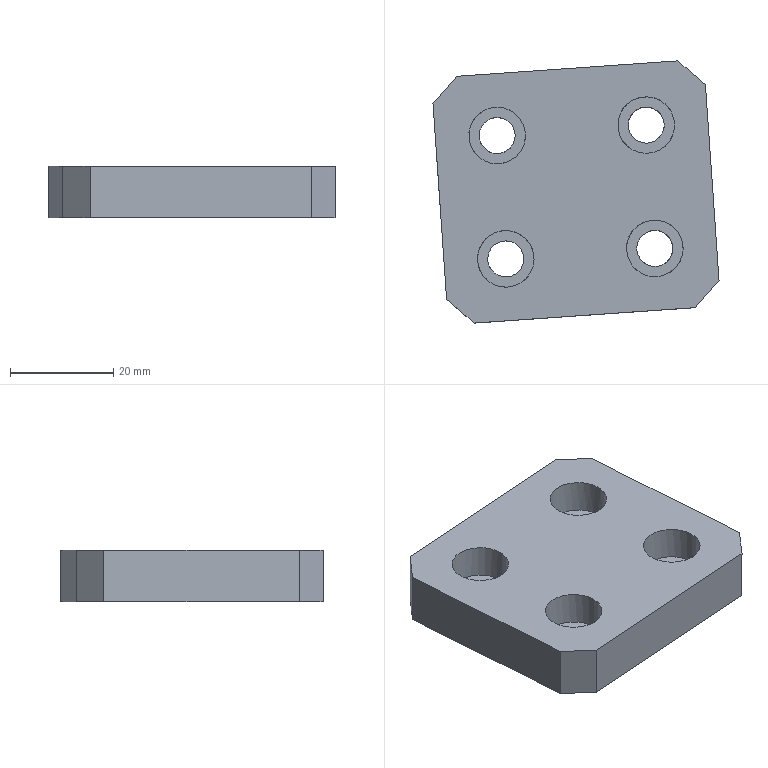Part | STEP file | 车灯-后视镜_id658_x_t | 1 solid | 22 faces | box 55.522 x 50.883 x 10 mm | volume 21930 mm3 | plane 14 | cylinder 8 | commonest cylinder face diameters 7 x4 11 x4
STEP:
#1=CARTESIAN_POINT('',(-17.129,7.094,-255.5));
#2=VERTEX_POINT('',#1);
#3=CARTESIAN_POINT('',(25.767,10.093,-255.5));
#4=VERTEX_POINT('',#3);
#5=CARTESIAN_POINT('',(3.398,8.529,-255.5));
#6=DIRECTION('',(0.9976,0.06976,0.));
#7=VECTOR('',#6,1.);
#8=LINE('',#5,#7);
#9=EDGE_CURVE('',#2,#4,#8,.T.);
#10=ORIENTED_EDGE('',*,*,#9,.F.);
#11=CARTESIAN_POINT('',(-21.768,1.757,-255.5));
#12=VERTEX_POINT('',#11);
#13=CARTESIAN_POINT('',(-26.608,-3.811,-255.5));
#14=DIRECTION('',(-0.6561,-0.7547,0.));
#15=VECTOR('',#14,1.);
#16=LINE('',#13,#15);
#17=EDGE_CURVE('',#2,#12,#16,.T.);
#18=ORIENTED_EDGE('',*,*,#17,.T.);
#19=CARTESIAN_POINT('',(-19.117,-36.15,-255.5));
#20=VERTEX_POINT('',#19);
#21=CARTESIAN_POINT('',(-19.256,-34.167,-255.5));
#22=DIRECTION('',(-0.06976,0.9976,0.));
#23=VECTOR('',#22,1.);
#24=LINE('',#21,#23);
#25=EDGE_CURVE('',#20,#12,#24,.T.);
#26=ORIENTED_EDGE('',*,*,#25,.F.);
#27=CARTESIAN_POINT('',(-13.78,-40.789,-255.5));
#28=VERTEX_POINT('',#27);
#29=CARTESIAN_POINT('',(-6.529,-47.093,-255.5));
#30=DIRECTION('',(0.7547,-0.6561,0.));
#31=VECTOR('',#30,1.);
#32=LINE('',#29,#31);
#33=EDGE_CURVE('',#20,#28,#32,.T.);
#34=ORIENTED_EDGE('',*,*,#33,.T.);
#35=CARTESIAN_POINT('',(29.115,-37.79,-255.5));
#36=VERTEX_POINT('',#35);
#37=CARTESIAN_POINT('',(6.747,-39.354,-255.5));
#38=DIRECTION('',(-0.9976,-0.06976,0.));
#39=VECTOR('',#38,1.);
#40=LINE('',#37,#39);
#41=EDGE_CURVE('',#36,#28,#40,.T.);
#42=ORIENTED_EDGE('',*,*,#41,.F.);
#43=CARTESIAN_POINT('',(33.754,-32.453,-255.5));
#44=VERTEX_POINT('',#43);
#45=CARTESIAN_POINT('',(21.955,-46.026,-255.5));
#46=DIRECTION('',(0.6561,0.7547,0.));
#47=VECTOR('',#46,1.);
#48=LINE('',#45,#47);
#49=EDGE_CURVE('',#36,#44,#48,.T.);
#50=ORIENTED_EDGE('',*,*,#49,.T.);
#51=CARTESIAN_POINT('',(31.103,5.454,-255.5));
#52=VERTEX_POINT('',#51);
#53=CARTESIAN_POINT('',(33.615,-30.47,-255.5));
#54=DIRECTION('',(0.06976,-0.9976,0.));
#55=VECTOR('',#54,1.);
#56=LINE('',#53,#55);
#57=EDGE_CURVE('',#52,#44,#56,.T.);
#58=ORIENTED_EDGE('',*,*,#57,.F.);
#59=CARTESIAN_POINT('',(35.687,1.47,-255.5));
#60=DIRECTION('',(-0.7547,0.6561,0.));
#61=VECTOR('',#60,1.);
#62=LINE('',#59,#61);
#63=EDGE_CURVE('',#52,#4,#62,.T.);
#64=ORIENTED_EDGE('',*,*,#63,.T.);
#65=EDGE_LOOP('',(#10,#18,#26,#34,#42,#50,#58,#64));
#66=FACE_BOUND('',#65,.T.);
#67=CARTESIAN_POINT('',(21.295,-31.807,-255.5));
#68=VERTEX_POINT('',#67);
#69=CARTESIAN_POINT('',(21.295,-26.307,-255.5));
#70=DIRECTION('',(0.,0.,1.));
#71=DIRECTION('',(0.,-1.,0.));
#72=AXIS2_PLACEMENT_3D('',#69,#70,#71);
#73=CIRCLE('',#72,5.5);
#74=EDGE_CURVE('',#68,#68,#73,.T.);
#75=ORIENTED_EDGE('',*,*,#74,.F.);
#76=EDGE_LOOP('',(#75));
#77=FACE_BOUND('',#76,.T.);
#78=CARTESIAN_POINT('',(19.621,-7.866,-255.5));
#79=VERTEX_POINT('',#78);
#80=CARTESIAN_POINT('',(19.621,-2.366,-255.5));
#81=DIRECTION('',(0.,0.,-1.));
#82=DIRECTION('',(0.,-1.,0.));
#83=AXIS2_PLACEMENT_3D('',#80,#81,#82);
#84=CIRCLE('',#83,5.5);
#85=EDGE_CURVE('',#79,#79,#84,.T.);
#86=ORIENTED_EDGE('',*,*,#85,.T.);
#87=EDGE_LOOP('',(#86));
#88=FACE_BOUND('',#87,.T.);
#89=CARTESIAN_POINT('',(-7.635,-33.83,-255.5));
#90=VERTEX_POINT('',#89);
#91=CARTESIAN_POINT('',(-7.635,-28.33,-255.5));
#92=DIRECTION('',(0.,0.,-1.));
#93=DIRECTION('',(0.,-1.,0.));
#94=AXIS2_PLACEMENT_3D('',#91,#92,#93);
#95=CIRCLE('',#94,5.5);
#96=EDGE_CURVE('',#90,#90,#95,.T.);
#97=ORIENTED_EDGE('',*,*,#96,.T.);
#98=EDGE_LOOP('',(#97));
#99=FACE_BOUND('',#98,.T.);
#100=CARTESIAN_POINT('',(-9.357,1.111,-255.5));
#101=VERTEX_POINT('',#100);
#102=CARTESIAN_POINT('',(-9.309,-4.389,-255.5));
#103=DIRECTION('',(0.,0.,1.));
#104=DIRECTION('',(-0.008727,1.,0.));
#105=AXIS2_PLACEMENT_3D('',#102,#103,#104);
#106=CIRCLE('',#105,5.5);
#107=EDGE_CURVE('',#101,#101,#106,.T.);
#108=ORIENTED_EDGE('',*,*,#107,.F.);
#109=EDGE_LOOP('',(#108));
#110=FACE_BOUND('',#109,.T.);
#111=CARTESIAN_POINT('',(6.259,-32.383,-255.5));
#112=DIRECTION('',(0.,0.,1.));
#113=DIRECTION('',(-0.06976,0.9976,0.));
#114=AXIS2_PLACEMENT_3D('',#111,#112,#113);
#115=PLANE('',#114);
#116=ADVANCED_FACE('',(#66,#77,#88,#99,#110),#115,.T.);
#117=CARTESIAN_POINT('',(33.754,-32.453,-265.5));
#118=VERTEX_POINT('',#117);
#119=CARTESIAN_POINT('',(31.103,5.454,-265.5));
#120=VERTEX_POINT('',#119);
#121=CARTESIAN_POINT('',(33.615,-30.47,-265.5));
#122=DIRECTION('',(-0.06976,0.9976,0.));
#123=VECTOR('',#122,1.);
#124=LINE('',#121,#123);
#125=EDGE_CURVE('',#118,#120,#124,.T.);
#126=ORIENTED_EDGE('',*,*,#125,.T.);
#127=CARTESIAN_POINT('',(31.103,5.454,-267.5));
#128=DIRECTION('',(0.,0.,1.));
#129=VECTOR('',#128,1.);
#130=LINE('',#127,#129);
#131=EDGE_CURVE('',#120,#52,#130,.T.);
#132=ORIENTED_EDGE('',*,*,#131,.T.);
#133=ORIENTED_EDGE('',*,*,#57,.T.);
#134=CARTESIAN_POINT('',(33.754,-32.453,-267.5));
#135=DIRECTION('',(0.,0.,-1.));
#136=VECTOR('',#135,1.);
#137=LINE('',#134,#136);
#138=EDGE_CURVE('',#44,#118,#137,.T.);
#139=ORIENTED_EDGE('',*,*,#138,.T.);
#140=EDGE_LOOP('',(#126,#132,#133,#139));
#141=FACE_OUTER_BOUND('',#140,.T.);
#142=CARTESIAN_POINT('',(33.615,-30.47,-267.5));
#143=DIRECTION('',(0.9976,0.06976,0.));
#144=DIRECTION('',(0.,0.,-1.));
#145=AXIS2_PLACEMENT_3D('',#142,#143,#144);
#146=PLANE('',#145);
#147=ADVANCED_FACE('',(#141),#146,.T.);
#148=ORIENTED_EDGE('',*,*,#25,.T.);
#149=CARTESIAN_POINT('',(-21.768,1.757,-265.5));
#150=VERTEX_POINT('',#149);
#151=CARTESIAN_POINT('',(-21.768,1.757,-267.5));
#152=DIRECTION('',(0.,0.,-1.));
#153=VECTOR('',#152,1.);
#154=LINE('',#151,#153);
#155=EDGE_CURVE('',#12,#150,#154,.T.);
#156=ORIENTED_EDGE('',*,*,#155,.T.);
#157=CARTESIAN_POINT('',(-19.117,-36.15,-265.5));
#158=VERTEX_POINT('',#157);
#159=CARTESIAN_POINT('',(-19.256,-34.167,-265.5));
#160=DIRECTION('',(0.06976,-0.9976,0.));
#161=VECTOR('',#160,1.);
#162=LINE('',#159,#161);
#163=EDGE_CURVE('',#150,#158,#162,.T.);
#164=ORIENTED_EDGE('',*,*,#163,.T.);
#165=CARTESIAN_POINT('',(-19.117,-36.15,-267.5));
#166=DIRECTION('',(0.,0.,1.));
#167=VECTOR('',#166,1.);
#168=LINE('',#165,#167);
#169=EDGE_CURVE('',#158,#20,#168,.T.);
#170=ORIENTED_EDGE('',*,*,#169,.T.);
#171=EDGE_LOOP('',(#148,#156,#164,#170));
#172=FACE_OUTER_BOUND('',#171,.T.);
#173=CARTESIAN_POINT('',(-19.256,-34.167,-267.5));
#174=DIRECTION('',(-0.9976,-0.06976,0.));
#175=DIRECTION('',(0.,0.,1.));
#176=AXIS2_PLACEMENT_3D('',#173,#174,#175);
#177=PLANE('',#176);
#178=ADVANCED_FACE('',(#172),#177,.T.);
#179=ORIENTED_EDGE('',*,*,#163,.F.);
#180=CARTESIAN_POINT('',(-17.129,7.094,-265.5));
#181=VERTEX_POINT('',#180);
#182=CARTESIAN_POINT('',(-26.608,-3.811,-265.5));
#183=DIRECTION('',(0.6561,0.7547,0.));
#184=VECTOR('',#183,1.);
#185=LINE('',#182,#184);
#186=EDGE_CURVE('',#150,#181,#185,.T.);
#187=ORIENTED_EDGE('',*,*,#186,.T.);
#188=CARTESIAN_POINT('',(25.767,10.093,-265.5));
#189=VERTEX_POINT('',#188);
#190=CARTESIAN_POINT('',(3.398,8.529,-265.5));
#191=DIRECTION('',(-0.9976,-0.06976,0.));
#192=VECTOR('',#191,1.);
#193=LINE('',#190,#192);
#194=EDGE_CURVE('',#189,#181,#193,.T.);
#195=ORIENTED_EDGE('',*,*,#194,.F.);
#196=CARTESIAN_POINT('',(35.687,1.47,-265.5));
#197=DIRECTION('',(0.7547,-0.6561,0.));
#198=VECTOR('',#197,1.);
#199=LINE('',#196,#198);
#200=EDGE_CURVE('',#189,#120,#199,.T.);
#201=ORIENTED_EDGE('',*,*,#200,.T.);
#202=ORIENTED_EDGE('',*,*,#125,.F.);
#203=CARTESIAN_POINT('',(29.115,-37.79,-265.5));
#204=VERTEX_POINT('',#203);
#205=CARTESIAN_POINT('',(21.955,-46.026,-265.5));
#206=DIRECTION('',(-0.6561,-0.7547,0.));
#207=VECTOR('',#206,1.);
#208=LINE('',#205,#207);
#209=EDGE_CURVE('',#118,#204,#208,.T.);
#210=ORIENTED_EDGE('',*,*,#209,.T.);
#211=CARTESIAN_POINT('',(-13.78,-40.789,-265.5));
#212=VERTEX_POINT('',#211);
#213=CARTESIAN_POINT('',(6.747,-39.354,-265.5));
#214=DIRECTION('',(0.9976,0.06976,0.));
#215=VECTOR('',#214,1.);
#216=LINE('',#213,#215);
#217=EDGE_CURVE('',#212,#204,#216,.T.);
#218=ORIENTED_EDGE('',*,*,#217,.F.);
#219=CARTESIAN_POINT('',(-6.529,-47.093,-265.5));
#220=DIRECTION('',(-0.7547,0.6561,0.));
#221=VECTOR('',#220,1.);
#222=LINE('',#219,#221);
#223=EDGE_CURVE('',#212,#158,#222,.T.);
#224=ORIENTED_EDGE('',*,*,#223,.T.);
#225=EDGE_LOOP('',(#179,#187,#195,#201,#202,#210,#218,#224));
#226=FACE_BOUND('',#225,.T.);
#227=CARTESIAN_POINT('',(21.295,-22.807,-265.5));
#228=VERTEX_POINT('',#227);
#229=CARTESIAN_POINT('',(21.295,-26.307,-265.5));
#230=DIRECTION('',(0.,0.,-1.));
#231=DIRECTION('',(0.,1.,0.));
#232=AXIS2_PLACEMENT_3D('',#229,#230,#231);
#233=CIRCLE('',#232,3.5);
#234=EDGE_CURVE('',#228,#228,#233,.T.);
#235=ORIENTED_EDGE('',*,*,#234,.F.);
#236=EDGE_LOOP('',(#235));
#237=FACE_BOUND('',#236,.T.);
#238=CARTESIAN_POINT('',(19.621,1.134,-265.5));
#239=VERTEX_POINT('',#238);
#240=CARTESIAN_POINT('',(19.621,-2.366,-265.5));
#241=DIRECTION('',(0.,0.,1.));
#242=DIRECTION('',(0.,1.,0.));
#243=AXIS2_PLACEMENT_3D('',#240,#241,#242);
#244=CIRCLE('',#243,3.5);
#245=EDGE_CURVE('',#239,#239,#244,.T.);
#246=ORIENTED_EDGE('',*,*,#245,.T.);
#247=EDGE_LOOP('',(#246));
#248=FACE_BOUND('',#247,.T.);
#249=CARTESIAN_POINT('',(-7.635,-24.83,-265.5));
#250=VERTEX_POINT('',#249);
#251=CARTESIAN_POINT('',(-7.635,-28.33,-265.5));
#252=DIRECTION('',(0.,0.,1.));
#253=DIRECTION('',(0.,1.,0.));
#254=AXIS2_PLACEMENT_3D('',#251,#252,#253);
#255=CIRCLE('',#254,3.5);
#256=EDGE_CURVE('',#250,#250,#255,.T.);
#257=ORIENTED_EDGE('',*,*,#256,.T.);
#258=EDGE_LOOP('',(#257));
#259=FACE_BOUND('',#258,.T.);
#260=CARTESIAN_POINT('',(-9.278,-7.888,-265.5));
#261=VERTEX_POINT('',#260);
#262=CARTESIAN_POINT('',(-9.309,-4.389,-265.5));
#263=DIRECTION('',(0.,0.,-1.));
#264=DIRECTION('',(0.008727,-1.,0.));
#265=AXIS2_PLACEMENT_3D('',#262,#263,#264);
#266=CIRCLE('',#265,3.5);
#267=EDGE_CURVE('',#261,#261,#266,.T.);
#268=ORIENTED_EDGE('',*,*,#267,.F.);
#269=EDGE_LOOP('',(#268));
#270=FACE_BOUND('',#269,.T.);
#271=CARTESIAN_POINT('',(6.259,-32.383,-265.5));
#272=DIRECTION('',(0.,0.,-1.));
#273=DIRECTION('',(0.06976,-0.9976,0.));
#274=AXIS2_PLACEMENT_3D('',#271,#272,#273);
#275=PLANE('',#274);
#276=ADVANCED_FACE('',(#226,#237,#248,#259,#270),#275,.T.);
#277=ORIENTED_EDGE('',*,*,#194,.T.);
#278=CARTESIAN_POINT('',(-17.129,7.094,-267.5));
#279=DIRECTION('',(0.,0.,1.));
#280=VECTOR('',#279,1.);
#281=LINE('',#278,#280);
#282=EDGE_CURVE('',#181,#2,#281,.T.);
#283=ORIENTED_EDGE('',*,*,#282,.T.);
#284=ORIENTED_EDGE('',*,*,#9,.T.);
#285=CARTESIAN_POINT('',(25.767,10.093,-267.5));
#286=DIRECTION('',(0.,0.,-1.));
#287=VECTOR('',#286,1.);
#288=LINE('',#285,#287);
#289=EDGE_CURVE('',#4,#189,#288,.T.);
#290=ORIENTED_EDGE('',*,*,#289,.T.);
#291=EDGE_LOOP('',(#277,#283,#284,#290));
#292=FACE_OUTER_BOUND('',#291,.T.);
#293=CARTESIAN_POINT('',(3.398,8.529,-267.5));
#294=DIRECTION('',(-0.06976,0.9976,0.));
#295=DIRECTION('',(0.,0.,-1.));
#296=AXIS2_PLACEMENT_3D('',#293,#294,#295);
#297=PLANE('',#296);
#298=ADVANCED_FACE('',(#292),#297,.T.);
#299=CARTESIAN_POINT('',(-9.065,-7.88,-262.));
#300=VERTEX_POINT('',#299);
#301=CARTESIAN_POINT('',(-9.309,-4.389,-262.));
#302=DIRECTION('',(0.,0.,-1.));
#303=DIRECTION('',(0.06976,-0.9976,0.));
#304=AXIS2_PLACEMENT_3D('',#301,#302,#303);
#305=CIRCLE('',#304,3.5);
#306=EDGE_CURVE('',#300,#300,#305,.T.);
#307=ORIENTED_EDGE('',*,*,#306,.F.);
#308=EDGE_LOOP('',(#307));
#309=FACE_BOUND('',#308,.T.);
#310=ORIENTED_EDGE('',*,*,#267,.T.);
#311=EDGE_LOOP('',(#310));
#312=FACE_BOUND('',#311,.T.);
#313=CARTESIAN_POINT('',(-9.309,-4.389,-265.5));
#314=DIRECTION('',(0.,0.,1.));
#315=DIRECTION('',(0.06976,-0.9976,0.));
#316=AXIS2_PLACEMENT_3D('',#313,#314,#315);
#317=CYLINDRICAL_SURFACE('',#316,3.5);
#318=ADVANCED_FACE('',(#309,#312),#317,.F.);
#319=ORIENTED_EDGE('',*,*,#306,.T.);
#320=EDGE_LOOP('',(#319));
#321=FACE_BOUND('',#320,.T.);
#322=CARTESIAN_POINT('',(-8.925,-9.875,-262.));
#323=VERTEX_POINT('',#322);
#324=CARTESIAN_POINT('',(-9.309,-4.389,-262.));
#325=DIRECTION('',(0.,0.,-1.));
#326=DIRECTION('',(0.06976,-0.9976,0.));
#327=AXIS2_PLACEMENT_3D('',#324,#325,#326);
#328=CIRCLE('',#327,5.5);
#329=EDGE_CURVE('',#323,#323,#328,.T.);
#330=ORIENTED_EDGE('',*,*,#329,.F.);
#331=EDGE_LOOP('',(#330));
#332=FACE_BOUND('',#331,.T.);
#333=CARTESIAN_POINT('',(-9.309,-4.389,-262.));
#334=DIRECTION('',(0.,0.,-1.));
#335=DIRECTION('',(-0.06976,0.9976,0.));
#336=AXIS2_PLACEMENT_3D('',#333,#334,#335);
#337=PLANE('',#336);
#338=ADVANCED_FACE('',(#321,#332),#337,.F.);
#339=ORIENTED_EDGE('',*,*,#329,.T.);
#340=EDGE_LOOP('',(#339));
#341=FACE_BOUND('',#340,.T.);
#342=ORIENTED_EDGE('',*,*,#107,.T.);
#343=EDGE_LOOP('',(#342));
#344=FACE_BOUND('',#343,.T.);
#345=CARTESIAN_POINT('',(-9.309,-4.389,-255.5));
#346=DIRECTION('',(0.,0.,-1.));
#347=DIRECTION('',(-0.06976,0.9976,0.));
#348=AXIS2_PLACEMENT_3D('',#345,#346,#347);
#349=CYLINDRICAL_SURFACE('',#348,5.5);
#350=ADVANCED_FACE('',(#341,#344),#349,.F.);
#351=CARTESIAN_POINT('',(-7.39,-31.822,-262.));
#352=VERTEX_POINT('',#351);
#353=CARTESIAN_POINT('',(-7.635,-28.33,-262.));
#354=DIRECTION('',(0.,0.,1.));
#355=DIRECTION('',(0.06976,-0.9976,0.));
#356=AXIS2_PLACEMENT_3D('',#353,#354,#355);
#357=CIRCLE('',#356,3.5);
#358=EDGE_CURVE('',#352,#352,#357,.T.);
#359=ORIENTED_EDGE('',*,*,#358,.T.);
#360=EDGE_LOOP('',(#359));
#361=FACE_BOUND('',#360,.T.);
#362=ORIENTED_EDGE('',*,*,#256,.F.);
#363=EDGE_LOOP('',(#362));
#364=FACE_BOUND('',#363,.T.);
#365=CARTESIAN_POINT('',(-7.635,-28.33,-265.5));
#366=DIRECTION('',(0.,0.,1.));
#367=DIRECTION('',(-0.06976,0.9976,0.));
#368=AXIS2_PLACEMENT_3D('',#365,#366,#367);
#369=CYLINDRICAL_SURFACE('',#368,3.5);
#370=ADVANCED_FACE('',(#361,#364),#369,.F.);
#371=ORIENTED_EDGE('',*,*,#358,.F.);
#372=EDGE_LOOP('',(#371));
#373=FACE_BOUND('',#372,.T.);
#374=CARTESIAN_POINT('',(-7.251,-33.817,-262.));
#375=VERTEX_POINT('',#374);
#376=CARTESIAN_POINT('',(-7.635,-28.33,-262.));
#377=DIRECTION('',(0.,0.,1.));
#378=DIRECTION('',(0.06976,-0.9976,0.));
#379=AXIS2_PLACEMENT_3D('',#376,#377,#378);
#380=CIRCLE('',#379,5.5);
#381=EDGE_CURVE('',#375,#375,#380,.T.);
#382=ORIENTED_EDGE('',*,*,#381,.T.);
#383=EDGE_LOOP('',(#382));
#384=FACE_BOUND('',#383,.T.);
#385=CARTESIAN_POINT('',(-7.635,-28.33,-262.));
#386=DIRECTION('',(0.,0.,-1.));
#387=DIRECTION('',(0.06976,-0.9976,0.));
#388=AXIS2_PLACEMENT_3D('',#385,#386,#387);
#389=PLANE('',#388);
#390=ADVANCED_FACE('',(#373,#384),#389,.F.);
#391=ORIENTED_EDGE('',*,*,#381,.F.);
#392=EDGE_LOOP('',(#391));
#393=FACE_BOUND('',#392,.T.);
#394=ORIENTED_EDGE('',*,*,#96,.F.);
#395=EDGE_LOOP('',(#394));
#396=FACE_BOUND('',#395,.T.);
#397=CARTESIAN_POINT('',(-7.635,-28.33,-255.5));
#398=DIRECTION('',(0.,0.,-1.));
#399=DIRECTION('',(0.06976,-0.9976,0.));
#400=AXIS2_PLACEMENT_3D('',#397,#398,#399);
#401=CYLINDRICAL_SURFACE('',#400,5.5);
#402=ADVANCED_FACE('',(#393,#396),#401,.F.);
#403=CARTESIAN_POINT('',(19.865,-5.857,-262.));
#404=VERTEX_POINT('',#403);
#405=CARTESIAN_POINT('',(19.621,-2.366,-262.));
#406=DIRECTION('',(0.,0.,1.));
#407=DIRECTION('',(0.06976,-0.9976,0.));
#408=AXIS2_PLACEMENT_3D('',#405,#406,#407);
#409=CIRCLE('',#408,3.5);
#410=EDGE_CURVE('',#404,#404,#409,.T.);
#411=ORIENTED_EDGE('',*,*,#410,.T.);
#412=EDGE_LOOP('',(#411));
#413=FACE_BOUND('',#412,.T.);
#414=ORIENTED_EDGE('',*,*,#245,.F.);
#415=EDGE_LOOP('',(#414));
#416=FACE_BOUND('',#415,.T.);
#417=CARTESIAN_POINT('',(19.621,-2.366,-265.5));
#418=DIRECTION('',(0.,0.,1.));
#419=DIRECTION('',(0.06976,-0.9976,0.));
#420=AXIS2_PLACEMENT_3D('',#417,#418,#419);
#421=CYLINDRICAL_SURFACE('',#420,3.5);
#422=ADVANCED_FACE('',(#413,#416),#421,.F.);
#423=ORIENTED_EDGE('',*,*,#410,.F.);
#424=EDGE_LOOP('',(#423));
#425=FACE_BOUND('',#424,.T.);
#426=CARTESIAN_POINT('',(20.004,-7.852,-262.));
#427=VERTEX_POINT('',#426);
#428=CARTESIAN_POINT('',(19.621,-2.366,-262.));
#429=DIRECTION('',(0.,0.,1.));
#430=DIRECTION('',(0.06976,-0.9976,0.));
#431=AXIS2_PLACEMENT_3D('',#428,#429,#430);
#432=CIRCLE('',#431,5.5);
#433=EDGE_CURVE('',#427,#427,#432,.T.);
#434=ORIENTED_EDGE('',*,*,#433,.T.);
#435=EDGE_LOOP('',(#434));
#436=FACE_BOUND('',#435,.T.);
#437=CARTESIAN_POINT('',(19.621,-2.366,-262.));
#438=DIRECTION('',(0.,0.,-1.));
#439=DIRECTION('',(-0.06976,0.9976,0.));
#440=AXIS2_PLACEMENT_3D('',#437,#438,#439);
#441=PLANE('',#440);
#442=ADVANCED_FACE('',(#425,#436),#441,.F.);
#443=ORIENTED_EDGE('',*,*,#433,.F.);
#444=EDGE_LOOP('',(#443));
#445=FACE_BOUND('',#444,.T.);
#446=ORIENTED_EDGE('',*,*,#85,.F.);
#447=EDGE_LOOP('',(#446));
#448=FACE_BOUND('',#447,.T.);
#449=CARTESIAN_POINT('',(19.621,-2.366,-255.5));
#450=DIRECTION('',(0.,0.,-1.));
#451=DIRECTION('',(-0.06976,0.9976,0.));
#452=AXIS2_PLACEMENT_3D('',#449,#450,#451);
#453=CYLINDRICAL_SURFACE('',#452,5.5);
#454=ADVANCED_FACE('',(#445,#448),#453,.F.);
#455=CARTESIAN_POINT('',(21.539,-29.799,-262.));
#456=VERTEX_POINT('',#455);
#457=CARTESIAN_POINT('',(21.295,-26.307,-262.));
#458=DIRECTION('',(0.,0.,-1.));
#459=DIRECTION('',(0.06976,-0.9976,0.));
#460=AXIS2_PLACEMENT_3D('',#457,#458,#459);
#461=CIRCLE('',#460,3.5);
#462=EDGE_CURVE('',#456,#456,#461,.T.);
#463=ORIENTED_EDGE('',*,*,#462,.F.);
#464=EDGE_LOOP('',(#463));
#465=FACE_BOUND('',#464,.T.);
#466=ORIENTED_EDGE('',*,*,#234,.T.);
#467=EDGE_LOOP('',(#466));
#468=FACE_BOUND('',#467,.T.);
#469=CARTESIAN_POINT('',(21.295,-26.307,-265.5));
#470=DIRECTION('',(0.,0.,1.));
#471=DIRECTION('',(-0.06976,0.9976,0.));
#472=AXIS2_PLACEMENT_3D('',#469,#470,#471);
#473=CYLINDRICAL_SURFACE('',#472,3.5);
#474=ADVANCED_FACE('',(#465,#468),#473,.F.);
#475=ORIENTED_EDGE('',*,*,#462,.T.);
#476=EDGE_LOOP('',(#475));
#477=FACE_BOUND('',#476,.T.);
#478=CARTESIAN_POINT('',(21.678,-31.794,-262.));
#479=VERTEX_POINT('',#478);
#480=CARTESIAN_POINT('',(21.295,-26.307,-262.));
#481=DIRECTION('',(0.,0.,-1.));
#482=DIRECTION('',(0.06976,-0.9976,0.));
#483=AXIS2_PLACEMENT_3D('',#480,#481,#482);
#484=CIRCLE('',#483,5.5);
#485=EDGE_CURVE('',#479,#479,#484,.T.);
#486=ORIENTED_EDGE('',*,*,#485,.F.);
#487=EDGE_LOOP('',(#486));
#488=FACE_BOUND('',#487,.T.);
#489=CARTESIAN_POINT('',(21.295,-26.307,-262.));
#490=DIRECTION('',(0.,0.,-1.));
#491=DIRECTION('',(0.06976,-0.9976,0.));
#492=AXIS2_PLACEMENT_3D('',#489,#490,#491);
#493=PLANE('',#492);
#494=ADVANCED_FACE('',(#477,#488),#493,.F.);
#495=ORIENTED_EDGE('',*,*,#485,.T.);
#496=EDGE_LOOP('',(#495));
#497=FACE_BOUND('',#496,.T.);
#498=ORIENTED_EDGE('',*,*,#74,.T.);
#499=EDGE_LOOP('',(#498));
#500=FACE_BOUND('',#499,.T.);
#501=CARTESIAN_POINT('',(21.295,-26.307,-255.5));
#502=DIRECTION('',(0.,0.,-1.));
#503=DIRECTION('',(0.06976,-0.9976,0.));
#504=AXIS2_PLACEMENT_3D('',#501,#502,#503);
#505=CYLINDRICAL_SURFACE('',#504,5.5);
#506=ADVANCED_FACE('',(#497,#500),#505,.F.);
#507=ORIENTED_EDGE('',*,*,#217,.T.);
#508=CARTESIAN_POINT('',(29.115,-37.79,-261.5));
#509=DIRECTION('',(0.,0.,1.));
#510=VECTOR('',#509,1.);
#511=LINE('',#508,#510);
#512=EDGE_CURVE('',#204,#36,#511,.T.);
#513=ORIENTED_EDGE('',*,*,#512,.T.);
#514=ORIENTED_EDGE('',*,*,#41,.T.);
#515=CARTESIAN_POINT('',(-13.78,-40.789,-261.5));
#516=DIRECTION('',(0.,0.,-1.));
#517=VECTOR('',#516,1.);
#518=LINE('',#515,#517);
#519=EDGE_CURVE('',#28,#212,#518,.T.);
#520=ORIENTED_EDGE('',*,*,#519,.T.);
#521=EDGE_LOOP('',(#507,#513,#514,#520));
#522=FACE_OUTER_BOUND('',#521,.T.);
#523=CARTESIAN_POINT('',(6.747,-39.354,-261.5));
#524=DIRECTION('',(-0.06976,0.9976,0.));
#525=DIRECTION('',(0.,0.,1.));
#526=AXIS2_PLACEMENT_3D('',#523,#524,#525);
#527=PLANE('',#526);
#528=ADVANCED_FACE('',(#522),#527,.F.);
#529=ORIENTED_EDGE('',*,*,#209,.F.);
#530=ORIENTED_EDGE('',*,*,#138,.F.);
#531=ORIENTED_EDGE('',*,*,#49,.F.);
#532=ORIENTED_EDGE('',*,*,#512,.F.);
#533=EDGE_LOOP('',(#529,#530,#531,#532));
#534=FACE_OUTER_BOUND('',#533,.T.);
#535=CARTESIAN_POINT('',(29.115,-37.79,-261.5));
#536=DIRECTION('',(0.7547,-0.6561,0.));
#537=DIRECTION('',(0.6561,0.7547,0.));
#538=AXIS2_PLACEMENT_3D('',#535,#536,#537);
#539=PLANE('',#538);
#540=ADVANCED_FACE('',(#534),#539,.T.);
#541=ORIENTED_EDGE('',*,*,#33,.F.);
#542=ORIENTED_EDGE('',*,*,#169,.F.);
#543=ORIENTED_EDGE('',*,*,#223,.F.);
#544=ORIENTED_EDGE('',*,*,#519,.F.);
#545=EDGE_LOOP('',(#541,#542,#543,#544));
#546=FACE_OUTER_BOUND('',#545,.T.);
#547=CARTESIAN_POINT('',(-13.78,-40.789,-261.5));
#548=DIRECTION('',(-0.6561,-0.7547,0.));
#549=DIRECTION('',(0.7547,-0.6561,0.));
#550=AXIS2_PLACEMENT_3D('',#547,#548,#549);
#551=PLANE('',#550);
#552=ADVANCED_FACE('',(#546),#551,.T.);
#553=ORIENTED_EDGE('',*,*,#17,.F.);
#554=ORIENTED_EDGE('',*,*,#282,.F.);
#555=ORIENTED_EDGE('',*,*,#186,.F.);
#556=ORIENTED_EDGE('',*,*,#155,.F.);
#557=EDGE_LOOP('',(#553,#554,#555,#556));
#558=FACE_OUTER_BOUND('',#557,.T.);
#559=CARTESIAN_POINT('',(-21.768,1.757,-267.5));
#560=DIRECTION('',(0.7547,-0.6561,0.));
#561=DIRECTION('',(0.6561,0.7547,0.));
#562=AXIS2_PLACEMENT_3D('',#559,#560,#561);
#563=PLANE('',#562);
#564=ADVANCED_FACE('',(#558),#563,.F.);
#565=ORIENTED_EDGE('',*,*,#63,.F.);
#566=ORIENTED_EDGE('',*,*,#131,.F.);
#567=ORIENTED_EDGE('',*,*,#200,.F.);
#568=ORIENTED_EDGE('',*,*,#289,.F.);
#569=EDGE_LOOP('',(#565,#566,#567,#568));
#570=FACE_OUTER_BOUND('',#569,.T.);
#571=CARTESIAN_POINT('',(25.767,10.093,-267.5));
#572=DIRECTION('',(-0.6561,-0.7547,0.));
#573=DIRECTION('',(0.7547,-0.6561,0.));
#574=AXIS2_PLACEMENT_3D('',#571,#572,#573);
#575=PLANE('',#574);
#576=ADVANCED_FACE('',(#570),#575,.F.);
#577=CLOSED_SHELL('',(#116,#147,#178,#276,#298,#318,#338,#350,#370,#390,#402,#422,#442,#454,#474,#494,#506,#528,#540,#552,#564,#576));
#578=MANIFOLD_SOLID_BREP('',#577);
#579=(LENGTH_UNIT()NAMED_UNIT(*)SI_UNIT(.MILLI.,.METRE.));
#580=UNCERTAINTY_MEASURE_WITH_UNIT(LENGTH_MEASURE(0.00002),#579,'','');
#581=(NAMED_UNIT(*)PLANE_ANGLE_UNIT()SI_UNIT($,.RADIAN.));
#582=PLANE_ANGLE_MEASURE_WITH_UNIT(PLANE_ANGLE_MEASURE(0.01745),#581);
#583=DIMENSIONAL_EXPONENTS(0.,0.,0.,0.,0.,0.,0.);
#584=(CONVERSION_BASED_UNIT('DEGREE',#582)NAMED_UNIT(#583)PLANE_ANGLE_UNIT());
#585=(NAMED_UNIT(*)SI_UNIT($,.STERADIAN.)SOLID_ANGLE_UNIT());
#586=(GEOMETRIC_REPRESENTATION_CONTEXT(3)GLOBAL_UNCERTAINTY_ASSIGNED_CONTEXT((#580))GLOBAL_UNIT_ASSIGNED_CONTEXT((#579,#584,#585))REPRESENTATION_CONTEXT('',''));
#587=ADVANCED_BREP_SHAPE_REPRESENTATION('',(#578),#586);